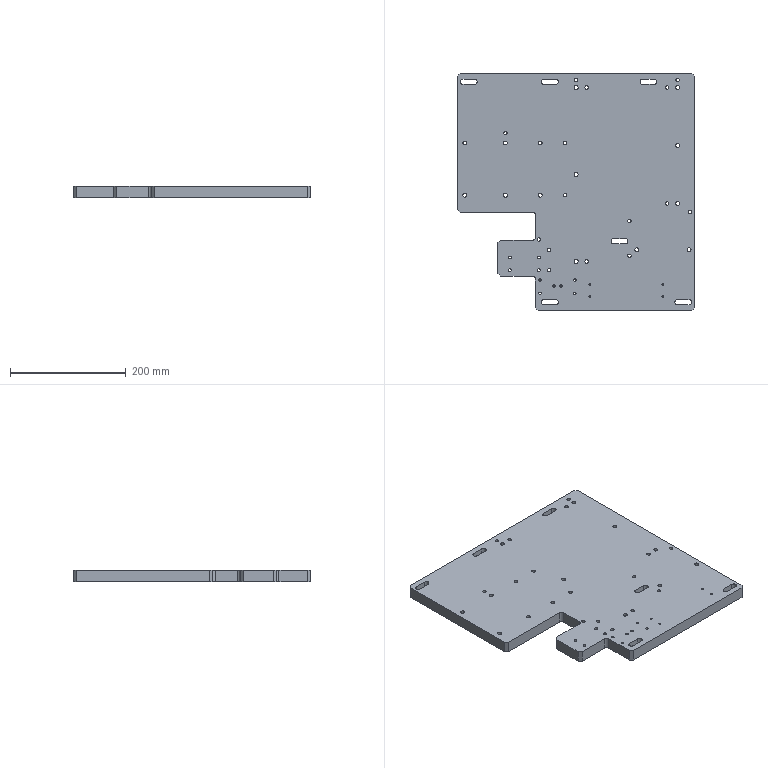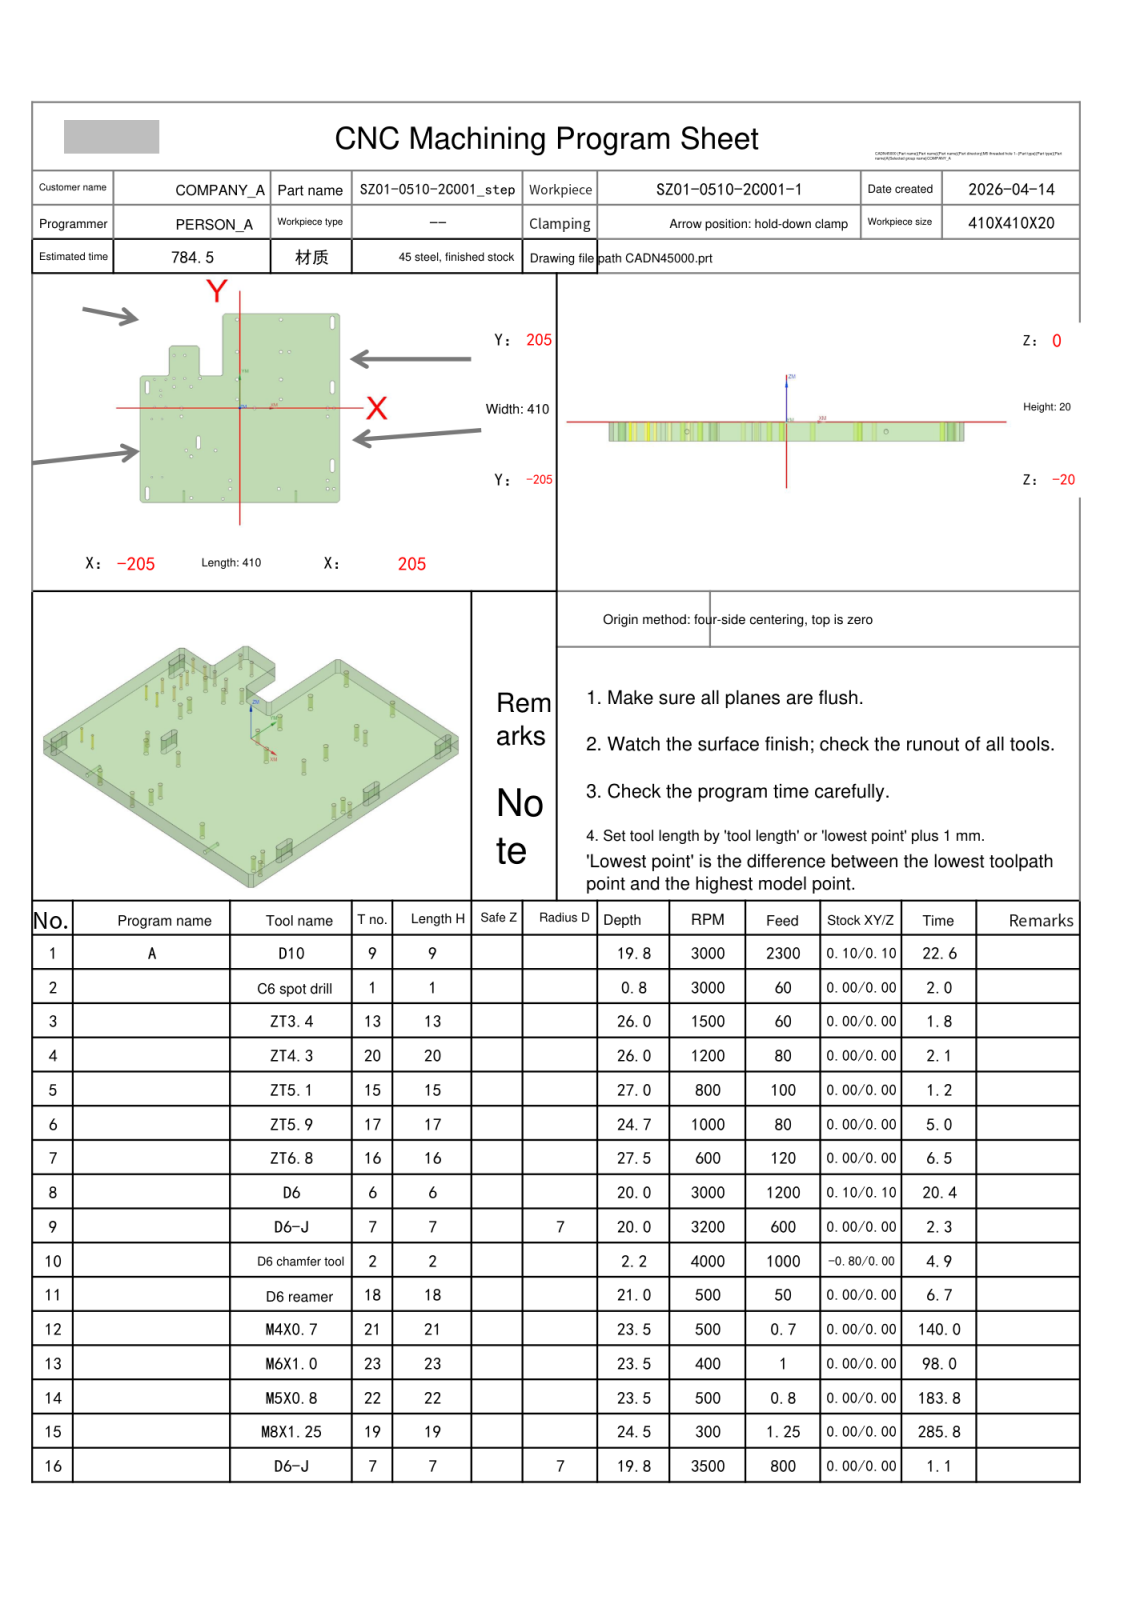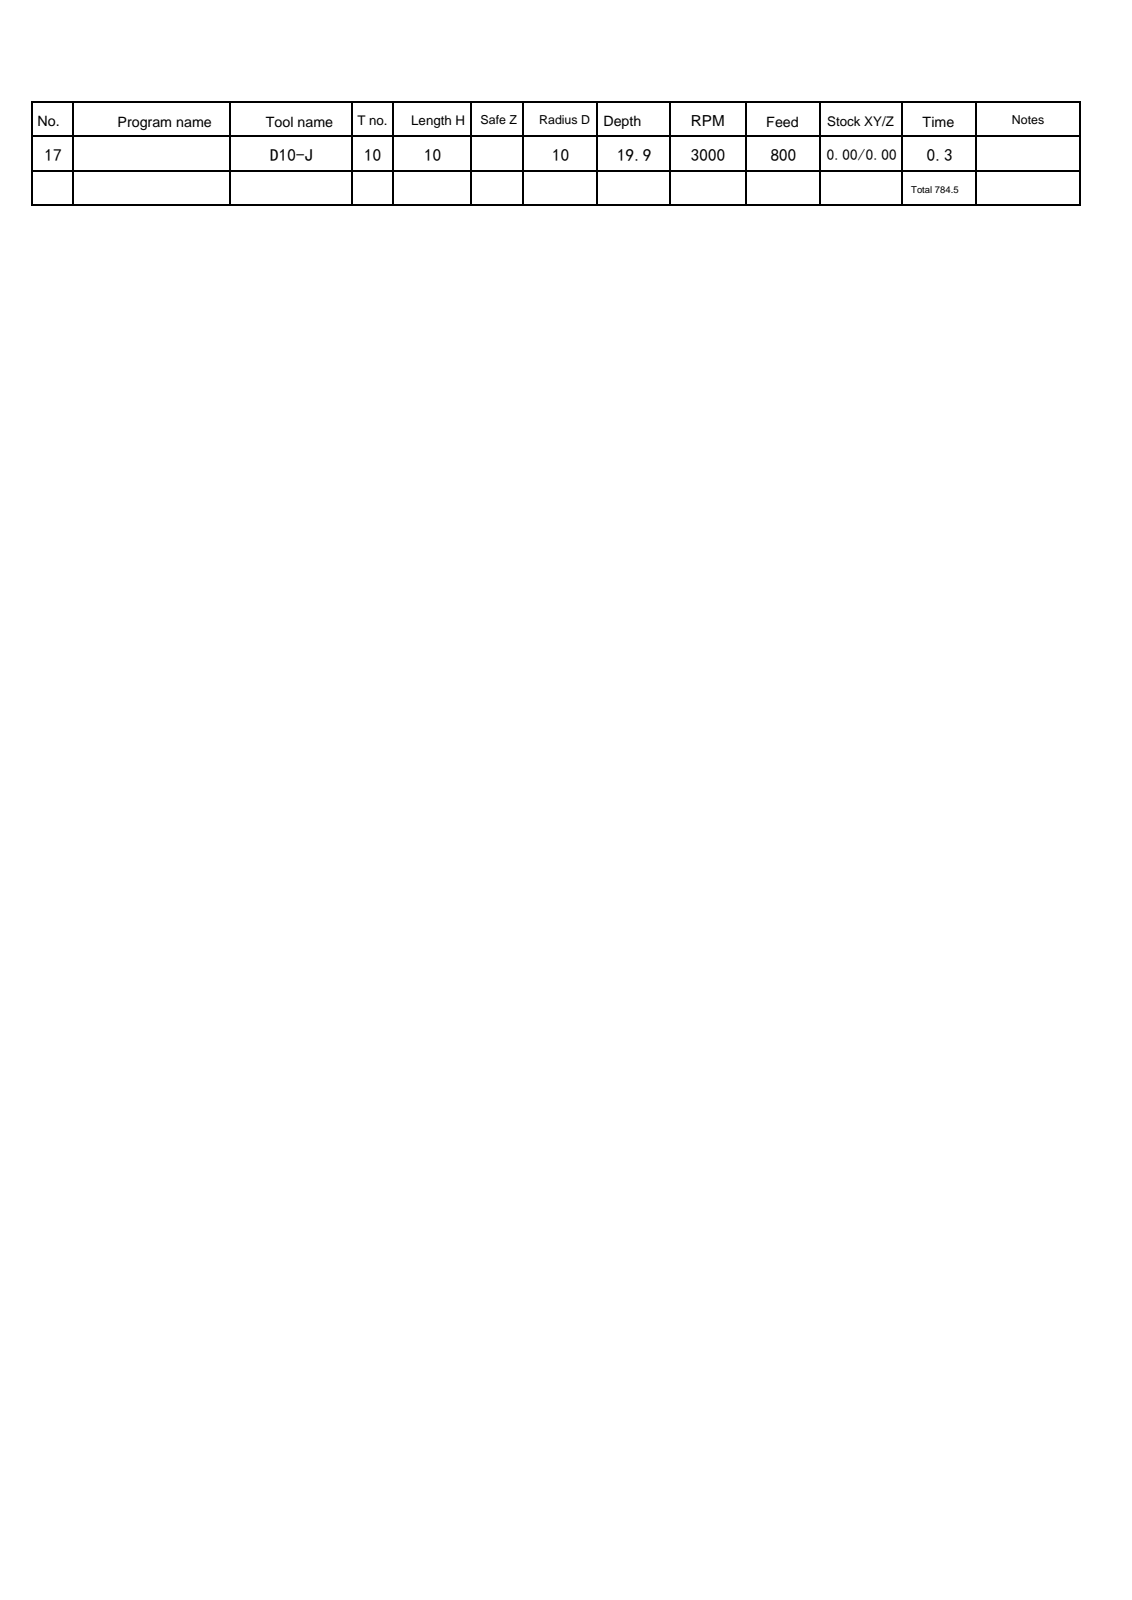NC program | NX | posted by the shop | part box 410 x 410 x 20 mm
Lines 26 to 1317 of 7905:
N1 T09 M06
(D10  D=10. R=0. H=09 ce=0.10 di=0.10)
G00 G90 G54 X215.1 Y-197.112 M03 S3000
G43 H09 Z50.
M08
Z-.2
G01 X208.606 Y-203.606 F2300.
X203.606 Y-208.606
X197.112 Y-215.1
G00 Z-.4
G01 X203.606 Y-208.606
X208.606 Y-203.606
X215.1 Y-197.112
G00 Z-.6
G01 X208.606 Y-203.606
X203.606 Y-208.606
X197.112 Y-215.1
G00 Z-.8
G01 X203.606 Y-208.606
X208.606 Y-203.606
X215.1 Y-197.112
G00 Z-1.
G01 X208.606 Y-203.606
X203.606 Y-208.606
X197.112 Y-215.1
G00 Z-1.2
G01 X203.606 Y-208.606
X208.606 Y-203.606
X215.1 Y-197.112
G00 Z-1.4
G01 X208.606 Y-203.606
X203.606 Y-208.606
X197.112 Y-215.1
G00 Z-1.6
G01 X203.606 Y-208.606
X208.606 Y-203.606
X215.1 Y-197.112
G00 Z-1.8
G01 X208.606 Y-203.606
X203.606 Y-208.606
X197.112 Y-215.1
G00 Z-2.
G01 X203.606 Y-208.606
X208.606 Y-203.606
X215.1 Y-197.112
G00 Z-2.2
G01 X208.606 Y-203.606
X203.606 Y-208.606
X197.112 Y-215.1
G00 Z-2.4
G01 X203.606 Y-208.606
X208.606 Y-203.606
X215.1 Y-197.112
G00 Z-2.6
G01 X208.606 Y-203.606
X203.606 Y-208.606
X197.112 Y-215.1
G00 Z-2.8
G01 X203.606 Y-208.606
X208.606 Y-203.606
X215.1 Y-197.112
G00 Z-3.
G01 X208.606 Y-203.606
X203.606 Y-208.606
X197.112 Y-215.1
G00 Z-3.2
G01 X203.606 Y-208.606
X208.606 Y-203.606
X215.1 Y-197.112
G00 Z-3.4
G01 X208.606 Y-203.606
X203.606 Y-208.606
X197.112 Y-215.1
G00 Z-3.6
G01 X203.606 Y-208.606
X208.606 Y-203.606
X215.1 Y-197.112
G00 Z-3.8
G01 X208.606 Y-203.606
X203.606 Y-208.606
X197.112 Y-215.1
G00 Z-4.
G01 X203.606 Y-208.606
X208.606 Y-203.606
X215.1 Y-197.112
G00 Z-4.2
G01 X208.606 Y-203.606
X203.606 Y-208.606
X197.112 Y-215.1
G00 Z-4.4
G01 X203.606 Y-208.606
X208.606 Y-203.606
X215.1 Y-197.112
G00 Z-4.6
G01 X208.606 Y-203.606
X203.606 Y-208.606
X197.112 Y-215.1
G00 Z-4.8
G01 X203.606 Y-208.606
X208.606 Y-203.606
X215.1 Y-197.112
G00 Z-5.
G01 X208.606 Y-203.606
X203.606 Y-208.606
X197.112 Y-215.1
G00 Z-5.2
G01 X203.606 Y-208.606
X208.606 Y-203.606
X215.1 Y-197.112
G00 Z-5.4
G01 X208.606 Y-203.606
X203.606 Y-208.606
X197.112 Y-215.1
G00 Z-5.6
G01 X203.606 Y-208.606
X208.606 Y-203.606
X215.1 Y-197.112
G00 Z-5.8
G01 X208.606 Y-203.606
X203.606 Y-208.606
X197.112 Y-215.1
G00 Z-6.
G01 X203.606 Y-208.606
X208.606 Y-203.606
X215.1 Y-197.112
G00 Z-6.2
G01 X208.606 Y-203.606
X203.606 Y-208.606
X197.112 Y-215.1
G00 Z-6.4
G01 X203.606 Y-208.606
X208.606 Y-203.606
X215.1 Y-197.112
G00 Z-6.6
G01 X208.606 Y-203.606
X203.606 Y-208.606
X197.112 Y-215.1
G00 Z-6.8
G01 X203.606 Y-208.606
X208.606 Y-203.606
X215.1 Y-197.112
G00 Z-7.
G01 X208.606 Y-203.606
X203.606 Y-208.606
X197.112 Y-215.1
G00 Z-7.2
G01 X203.606 Y-208.606
X208.606 Y-203.606
X215.1 Y-197.112
G00 Z-7.4
G01 X208.606 Y-203.606
X203.606 Y-208.606
X197.112 Y-215.1
G00 Z-7.6
G01 X203.606 Y-208.606
X208.606 Y-203.606
X215.1 Y-197.112
G00 Z-7.8
G01 X208.606 Y-203.606
X203.606 Y-208.606
X197.112 Y-215.1
G00 Z-8.
G01 X203.606 Y-208.606
X208.606 Y-203.606
X215.1 Y-197.112
G00 Z-8.2
G01 X208.606 Y-203.606
X203.606 Y-208.606
X197.112 Y-215.1
G00 Z-8.4
G01 X203.606 Y-208.606
X208.606 Y-203.606
X215.1 Y-197.112
G00 Z-8.6
G01 X208.606 Y-203.606
X203.606 Y-208.606
X197.112 Y-215.1
G00 Z-8.8
G01 X203.606 Y-208.606
X208.606 Y-203.606
X215.1 Y-197.112
G00 Z-9.
G01 X208.606 Y-203.606
X203.606 Y-208.606
X197.112 Y-215.1
G00 Z-9.2
G01 X203.606 Y-208.606
X208.606 Y-203.606
X215.1 Y-197.112
G00 Z-9.4
G01 X208.606 Y-203.606
X203.606 Y-208.606
X197.112 Y-215.1
G00 Z-9.6
G01 X203.606 Y-208.606
X208.606 Y-203.606
X215.1 Y-197.112
G00 Z-9.8
G01 X208.606 Y-203.606
X203.606 Y-208.606
X197.112 Y-215.1
G00 Z-10.
G01 X203.606 Y-208.606
X208.606 Y-203.606
X215.1 Y-197.112
G00 Z-10.2
G01 X208.606 Y-203.606
X203.606 Y-208.606
X197.112 Y-215.1
G00 Z-10.4
G01 X203.606 Y-208.606
X208.606 Y-203.606
X215.1 Y-197.112
G00 Z-10.6
G01 X208.606 Y-203.606
X203.606 Y-208.606
X197.112 Y-215.1
G00 Z-10.8
G01 X203.606 Y-208.606
X208.606 Y-203.606
X215.1 Y-197.112
G00 Z-11.
G01 X208.606 Y-203.606
X203.606 Y-208.606
X197.112 Y-215.1
G00 Z-11.2
G01 X203.606 Y-208.606
X208.606 Y-203.606
X215.1 Y-197.112
G00 Z-11.4
G01 X208.606 Y-203.606
X203.606 Y-208.606
X197.112 Y-215.1
G00 Z-11.6
G01 X203.606 Y-208.606
X208.606 Y-203.606
X215.1 Y-197.112
G00 Z-11.8
G01 X208.606 Y-203.606
X203.606 Y-208.606
X197.112 Y-215.1
G00 Z-12.
G01 X203.606 Y-208.606
X208.606 Y-203.606
X215.1 Y-197.112
G00 Z-12.2
G01 X208.606 Y-203.606
X203.606 Y-208.606
X197.112 Y-215.1
G00 Z-12.4
G01 X203.606 Y-208.606
X208.606 Y-203.606
X215.1 Y-197.112
G00 Z-12.6
G01 X208.606 Y-203.606
X203.606 Y-208.606
X197.112 Y-215.1
G00 Z-12.8
G01 X203.606 Y-208.606
X208.606 Y-203.606
X215.1 Y-197.112
G00 Z-13.
G01 X208.606 Y-203.606
X203.606 Y-208.606
X197.112 Y-215.1
G00 Z-13.2
G01 X203.606 Y-208.606
X208.606 Y-203.606
X215.1 Y-197.112
G00 Z-13.4
G01 X208.606 Y-203.606
X203.606 Y-208.606
X197.112 Y-215.1
G00 Z-13.6
G01 X203.606 Y-208.606
X208.606 Y-203.606
X215.1 Y-197.112
G00 Z-13.8
G01 X208.606 Y-203.606
X203.606 Y-208.606
X197.112 Y-215.1
G00 Z-14.
G01 X203.606 Y-208.606
X208.606 Y-203.606
X215.1 Y-197.112
G00 Z-14.2
G01 X208.606 Y-203.606
X203.606 Y-208.606
X197.112 Y-215.1
G00 Z-14.4
G01 X203.606 Y-208.606
X208.606 Y-203.606
X215.1 Y-197.112
G00 Z-14.6
G01 X208.606 Y-203.606
X203.606 Y-208.606
X197.112 Y-215.1
G00 Z-14.8
G01 X203.606 Y-208.606
X208.606 Y-203.606
X215.1 Y-197.112
G00 Z-15.
G01 X208.606 Y-203.606
X203.606 Y-208.606
X197.112 Y-215.1
G00 Z-15.2
G01 X203.606 Y-208.606
X208.606 Y-203.606
X215.1 Y-197.112
G00 Z-15.4
G01 X208.606 Y-203.606
X203.606 Y-208.606
X197.112 Y-215.1
G00 Z-15.6
G01 X203.606 Y-208.606
X208.606 Y-203.606
X215.1 Y-197.112
G00 Z-15.8
G01 X208.606 Y-203.606
X203.606 Y-208.606
X197.112 Y-215.1
G00 Z-16.
G01 X203.606 Y-208.606
X208.606 Y-203.606
X215.1 Y-197.112
G00 Z-16.2
G01 X208.606 Y-203.606
X203.606 Y-208.606
X197.112 Y-215.1
G00 Z-16.4
G01 X203.606 Y-208.606
X208.606 Y-203.606
X215.1 Y-197.112
G00 Z-16.6
G01 X208.606 Y-203.606
X203.606 Y-208.606
X197.112 Y-215.1
G00 Z-16.8
G01 X203.606 Y-208.606
X208.606 Y-203.606
X215.1 Y-197.112
G00 Z-17.
G01 X208.606 Y-203.606
X203.606 Y-208.606
X197.112 Y-215.1
G00 Z-17.2
G01 X203.606 Y-208.606
X208.606 Y-203.606
X215.1 Y-197.112
G00 Z-17.4
G01 X208.606 Y-203.606
X203.606 Y-208.606
X197.112 Y-215.1
G00 Z-17.6
G01 X203.606 Y-208.606
X208.606 Y-203.606
X215.1 Y-197.112
G00 Z-17.8
G01 X208.606 Y-203.606
X203.606 Y-208.606
X197.112 Y-215.1
G00 Z-18.
G01 X203.606 Y-208.606
X208.606 Y-203.606
X215.1 Y-197.112
G00 Z-18.2
G01 X208.606 Y-203.606
X203.606 Y-208.606
X197.112 Y-215.1
G00 Z-18.4
G01 X203.606 Y-208.606
X208.606 Y-203.606
X215.1 Y-197.112
G00 Z-18.6
G01 X208.606 Y-203.606
X203.606 Y-208.606
X197.112 Y-215.1
G00 Z-18.8
G01 X203.606 Y-208.606
X208.606 Y-203.606
X215.1 Y-197.112
G00 Z-19.
G01 X208.606 Y-203.606
X203.606 Y-208.606
X197.112 Y-215.1
G00 Z-19.2
G01 X203.606 Y-208.606
X208.606 Y-203.606
X215.1 Y-197.112
G00 Z-19.4
G01 X208.606 Y-203.606
X203.606 Y-208.606
X197.112 Y-215.1
G00 Z-19.6
G01 X203.606 Y-208.606
X208.606 Y-203.606
X215.1 Y-197.112
G00 Z-19.8
G01 X208.606 Y-203.606
X203.606 Y-208.606
X197.112 Y-215.1
G00 Z50.
X-197.112
Z-.2
G01 X-203.606 Y-208.606
X-208.606 Y-203.606
X-215.1 Y-197.112
G00 Z-.4
G01 X-208.606 Y-203.606
X-203.606 Y-208.606
X-197.112 Y-215.1
G00 Z-.6
G01 X-203.606 Y-208.606
X-208.606 Y-203.606
X-215.1 Y-197.112
G00 Z-.8
G01 X-208.606 Y-203.606
X-203.606 Y-208.606
X-197.112 Y-215.1
G00 Z-1.
G01 X-203.606 Y-208.606
X-208.606 Y-203.606
X-215.1 Y-197.112
G00 Z-1.2
G01 X-208.606 Y-203.606
X-203.606 Y-208.606
X-197.112 Y-215.1
G00 Z-1.4
G01 X-203.606 Y-208.606
X-208.606 Y-203.606
X-215.1 Y-197.112
G00 Z-1.6
G01 X-208.606 Y-203.606
X-203.606 Y-208.606
X-197.112 Y-215.1
G00 Z-1.8
G01 X-203.606 Y-208.606
X-208.606 Y-203.606
X-215.1 Y-197.112
G00 Z-2.
G01 X-208.606 Y-203.606
X-203.606 Y-208.606
X-197.112 Y-215.1
G00 Z-2.2
G01 X-203.606 Y-208.606
X-208.606 Y-203.606
X-215.1 Y-197.112
G00 Z-2.4
G01 X-208.606 Y-203.606
X-203.606 Y-208.606
X-197.112 Y-215.1
G00 Z-2.6
G01 X-203.606 Y-208.606
X-208.606 Y-203.606
X-215.1 Y-197.112
G00 Z-2.8
G01 X-208.606 Y-203.606
X-203.606 Y-208.606
X-197.112 Y-215.1
G00 Z-3.
G01 X-203.606 Y-208.606
X-208.606 Y-203.606
X-215.1 Y-197.112
G00 Z-3.2
G01 X-208.606 Y-203.606
X-203.606 Y-208.606
X-197.112 Y-215.1
G00 Z-3.4
G01 X-203.606 Y-208.606
X-208.606 Y-203.606
X-215.1 Y-197.112
G00 Z-3.6
G01 X-208.606 Y-203.606
X-203.606 Y-208.606
X-197.112 Y-215.1
G00 Z-3.8
G01 X-203.606 Y-208.606
X-208.606 Y-203.606
X-215.1 Y-197.112
G00 Z-4.
G01 X-208.606 Y-203.606
X-203.606 Y-208.606
X-197.112 Y-215.1
G00 Z-4.2
G01 X-203.606 Y-208.606
X-208.606 Y-203.606
X-215.1 Y-197.112
G00 Z-4.4
G01 X-208.606 Y-203.606
X-203.606 Y-208.606
X-197.112 Y-215.1
G00 Z-4.6
G01 X-203.606 Y-208.606
X-208.606 Y-203.606
X-215.1 Y-197.112
G00 Z-4.8
G01 X-208.606 Y-203.606
X-203.606 Y-208.606
X-197.112 Y-215.1
G00 Z-5.
G01 X-203.606 Y-208.606
X-208.606 Y-203.606
X-215.1 Y-197.112
G00 Z-5.2
G01 X-208.606 Y-203.606
X-203.606 Y-208.606
X-197.112 Y-215.1
G00 Z-5.4
G01 X-203.606 Y-208.606
X-208.606 Y-203.606
X-215.1 Y-197.112
G00 Z-5.6
G01 X-208.606 Y-203.606
X-203.606 Y-208.606
X-197.112 Y-215.1
G00 Z-5.8
G01 X-203.606 Y-208.606
X-208.606 Y-203.606
X-215.1 Y-197.112
G00 Z-6.
G01 X-208.606 Y-203.606
X-203.606 Y-208.606
X-197.112 Y-215.1
G00 Z-6.2
G01 X-203.606 Y-208.606
X-208.606 Y-203.606
X-215.1 Y-197.112
G00 Z-6.4
G01 X-208.606 Y-203.606
X-203.606 Y-208.606
X-197.112 Y-215.1
G00 Z-6.6
G01 X-203.606 Y-208.606
X-208.606 Y-203.606
X-215.1 Y-197.112
G00 Z-6.8
G01 X-208.606 Y-203.606
X-203.606 Y-208.606
X-197.112 Y-215.1
G00 Z-7.
G01 X-203.606 Y-208.606
X-208.606 Y-203.606
X-215.1 Y-197.112
G00 Z-7.2
G01 X-208.606 Y-203.606
X-203.606 Y-208.606
X-197.112 Y-215.1
G00 Z-7.4
G01 X-203.606 Y-208.606
X-208.606 Y-203.606
X-215.1 Y-197.112
G00 Z-7.6
G01 X-208.606 Y-203.606
X-203.606 Y-208.606
X-197.112 Y-215.1
G00 Z-7.8
G01 X-203.606 Y-208.606
X-208.606 Y-203.606
X-215.1 Y-197.112
G00 Z-8.
G01 X-208.606 Y-203.606
X-203.606 Y-208.606
X-197.112 Y-215.1
G00 Z-8.2
G01 X-203.606 Y-208.606
X-208.606 Y-203.606
X-215.1 Y-197.112
G00 Z-8.4
G01 X-208.606 Y-203.606
X-203.606 Y-208.606
X-197.112 Y-215.1
G00 Z-8.6
G01 X-203.606 Y-208.606
X-208.606 Y-203.606
X-215.1 Y-197.112
G00 Z-8.8
G01 X-208.606 Y-203.606
X-203.606 Y-208.606
X-197.112 Y-215.1
G00 Z-9.
G01 X-203.606 Y-208.606
X-208.606 Y-203.606
X-215.1 Y-197.112
G00 Z-9.2
G01 X-208.606 Y-203.606
X-203.606 Y-208.606
X-197.112 Y-215.1
G00 Z-9.4
G01 X-203.606 Y-208.606
X-208.606 Y-203.606
X-215.1 Y-197.112
G00 Z-9.6
G01 X-208.606 Y-203.606
X-203.606 Y-208.606
X-197.112 Y-215.1
G00 Z-9.8
G01 X-203.606 Y-208.606
X-208.606 Y-203.606
X-215.1 Y-197.112
G00 Z-10.
G01 X-208.606 Y-203.606
X-203.606 Y-208.606
X-197.112 Y-215.1
G00 Z-10.2
G01 X-203.606 Y-208.606
X-208.606 Y-203.606
X-215.1 Y-197.112
G00 Z-10.4
G01 X-208.606 Y-203.606
X-203.606 Y-208.606
X-197.112 Y-215.1
G00 Z-10.6
G01 X-203.606 Y-208.606
X-208.606 Y-203.606
X-215.1 Y-197.112
G00 Z-10.8
G01 X-208.606 Y-203.606
X-203.606 Y-208.606
X-197.112 Y-215.1
G00 Z-11.
G01 X-203.606 Y-208.606
X-208.606 Y-203.606
X-215.1 Y-197.112
G00 Z-11.2
G01 X-208.606 Y-203.606
X-203.606 Y-208.606
X-197.112 Y-215.1
G00 Z-11.4
G01 X-203.606 Y-208.606
X-208.606 Y-203.606
X-215.1 Y-197.112
G00 Z-11.6
G01 X-208.606 Y-203.606
X-203.606 Y-208.606
X-197.112 Y-215.1
G00 Z-11.8
G01 X-203.606 Y-208.606
X-208.606 Y-203.606
X-215.1 Y-197.112
G00 Z-12.
G01 X-208.606 Y-203.606
X-203.606 Y-208.606
X-197.112 Y-215.1
G00 Z-12.2
G01 X-203.606 Y-208.606
X-208.606 Y-203.606
X-215.1 Y-197.112
G00 Z-12.4
G01 X-208.606 Y-203.606
X-203.606 Y-208.606
X-197.112 Y-215.1
G00 Z-12.6
G01 X-203.606 Y-208.606
X-208.606 Y-203.606
X-215.1 Y-197.112
G00 Z-12.8
G01 X-208.606 Y-203.606
X-203.606 Y-208.606
X-197.112 Y-215.1
G00 Z-13.
G01 X-203.606 Y-208.606
X-208.606 Y-203.606
X-215.1 Y-197.112
G00 Z-13.2
G01 X-208.606 Y-203.606
X-203.606 Y-208.606
X-197.112 Y-215.1
G00 Z-13.4
G01 X-203.606 Y-208.606
X-208.606 Y-203.606
X-215.1 Y-197.112
G00 Z-13.6
G01 X-208.606 Y-203.606
X-203.606 Y-208.606
X-197.112 Y-215.1
G00 Z-13.8
G01 X-203.606 Y-208.606
X-208.606 Y-203.606
X-215.1 Y-197.112
G00 Z-14.
G01 X-208.606 Y-203.606
X-203.606 Y-208.606
X-197.112 Y-215.1
G00 Z-14.2
G01 X-203.606 Y-208.606
X-208.606 Y-203.606
X-215.1 Y-197.112
G00 Z-14.4
G01 X-208.606 Y-203.606
X-203.606 Y-208.606
X-197.112 Y-215.1
G00 Z-14.6
G01 X-203.606 Y-208.606
X-208.606 Y-203.606
X-215.1 Y-197.112
G00 Z-14.8
G01 X-208.606 Y-203.606
X-203.606 Y-208.606
X-197.112 Y-215.1
G00 Z-15.
G01 X-203.606 Y-208.606
X-208.606 Y-203.606
X-215.1 Y-197.112
G00 Z-15.2
G01 X-208.606 Y-203.606
X-203.606 Y-208.606
X-197.112 Y-215.1
G00 Z-15.4
G01 X-203.606 Y-208.606
X-208.606 Y-203.606
X-215.1 Y-197.112
G00 Z-15.6
G01 X-208.606 Y-203.606
X-203.606 Y-208.606
X-197.112 Y-215.1
G00 Z-15.8
G01 X-203.606 Y-208.606
X-208.606 Y-203.606
X-215.1 Y-197.112
G00 Z-16.
G01 X-208.606 Y-203.606
X-203.606 Y-208.606
X-197.112 Y-215.1
G00 Z-16.2
G01 X-203.606 Y-208.606
X-208.606 Y-203.606
X-215.1 Y-197.112
G00 Z-16.4
G01 X-208.606 Y-203.606
X-203.606 Y-208.606
X-197.112 Y-215.1
G00 Z-16.6
G01 X-203.606 Y-208.606
X-208.606 Y-203.606
X-215.1 Y-197.112
G00 Z-16.8
G01 X-208.606 Y-203.606
X-203.606 Y-208.606
X-197.112 Y-215.1
G00 Z-17.
G01 X-203.606 Y-208.606
X-208.606 Y-203.606
X-215.1 Y-197.112
G00 Z-17.2
G01 X-208.606 Y-203.606
X-203.606 Y-208.606
X-197.112 Y-215.1
G00 Z-17.4
G01 X-203.606 Y-208.606
X-208.606 Y-203.606
X-215.1 Y-197.112
G00 Z-17.6
G01 X-208.606 Y-203.606
X-203.606 Y-208.606
X-197.112 Y-215.1
G00 Z-17.8
G01 X-203.606 Y-208.606
X-208.606 Y-203.606
X-215.1 Y-197.112
G00 Z-18.
G01 X-208.606 Y-203.606
X-203.606 Y-208.606
X-197.112 Y-215.1
G00 Z-18.2
G01 X-203.606 Y-208.606
X-208.606 Y-203.606
X-215.1 Y-197.112
G00 Z-18.4
G01 X-208.606 Y-203.606
X-203.606 Y-208.606
X-197.112 Y-215.1
G00 Z-18.6
G01 X-203.606 Y-208.606
X-208.606 Y-203.606
X-215.1 Y-197.112
G00 Z-18.8
G01 X-208.606 Y-203.606
X-203.606 Y-208.606
X-197.112 Y-215.1
G00 Z-19.
G01 X-203.606 Y-208.606
X-208.606 Y-203.606
X-215.1 Y-197.112
G00 Z-19.2
G01 X-208.606 Y-203.606
X-203.606 Y-208.606
X-197.112 Y-215.1
G00 Z-19.4
G01 X-203.606 Y-208.606
X-208.606 Y-203.606
X-215.1 Y-197.112
G00 Z-19.6
G01 X-208.606 Y-203.606
X-203.606 Y-208.606
X-197.112 Y-215.1
G00 Z-19.8
G01 X-203.606 Y-208.606
X-208.606 Y-203.606
X-215.1 Y-197.112
G00 Z50.
Y62.112
Z-.2
G01 X-208.606 Y68.606
X-203.606 Y73.606
G02 X-200. Y75.1 I3.606 J-3.606
G01 X-150.1
Y130.
G02 X-148.606 Y133.606 I5.1 J0.0
G01 X-143.606 Y138.606
G02 X-140. Y140.1 I3.606 J-3.606
G01 X-88.
G02 X-84.394 Y138.606 I0.0 J-5.1
G01 X-79.394 Y133.606
G02 X-77.9 Y130. I-3.606 J-3.606
G01 Y75.1
X-40.1
Y200.
G02 X-38.606 Y203.606 I5.1 J0.0
G01 X-33.606 Y208.606
X-27.112 Y215.1
G00 Z-.4
G01 X-33.606 Y208.606
X-38.606 Y203.606
G03 X-40.1 Y200. I3.606 J-3.606
G01 Y75.1
X-77.9
Y130.
G03 X-79.394 Y133.606 I-5.1 J0.0
G01 X-84.394 Y138.606
G03 X-88. Y140.1 I-3.606 J-3.606
G01 X-140.
G03 X-143.606 Y138.606 I0.0 J-5.1
G01 X-148.606 Y133.606
G03 X-150.1 Y130. I3.606 J-3.606
G01 Y75.1
X-200.
G03 X-203.606 Y73.606 I0.0 J-5.1
G01 X-208.606 Y68.606
X-215.1 Y62.112
G00 Z-.6
G01 X-208.606 Y68.606
X-203.606 Y73.606
G02 X-200. Y75.1 I3.606 J-3.606
G01 X-150.1
Y130.
G02 X-148.606 Y133.606 I5.1 J0.0
G01 X-143.606 Y138.606
G02 X-140. Y140.1 I3.606 J-3.606
G01 X-88.
G02 X-84.394 Y138.606 I0.0 J-5.1
G01 X-79.394 Y133.606
G02 X-77.9 Y130. I-3.606 J-3.606
G01 Y75.1
X-40.1
Y200.
G02 X-38.606 Y203.606 I5.1 J0.0
G01 X-33.606 Y208.606
X-27.112 Y215.1
G00 Z-.8
G01 X-33.606 Y208.606
X-38.606 Y203.606
G03 X-40.1 Y200. I3.606 J-3.606
G01 Y75.1
X-77.9
Y130.
G03 X-79.394 Y133.606 I-5.1 J0.0
G01 X-84.394 Y138.606
G03 X-88. Y140.1 I-3.606 J-3.606
G01 X-140.
G03 X-143.606 Y138.606 I0.0 J-5.1
G01 X-148.606 Y133.606
G03 X-150.1 Y130. I3.606 J-3.606
G01 Y75.1
X-200.
G03 X-203.606 Y73.606 I0.0 J-5.1
G01 X-208.606 Y68.606
X-215.1 Y62.112
G00 Z-1.
G01 X-208.606 Y68.606
X-203.606 Y73.606
G02 X-200. Y75.1 I3.606 J-3.606
G01 X-150.1
Y130.
G02 X-148.606 Y133.606 I5.1 J0.0
G01 X-143.606 Y138.606
G02 X-140. Y140.1 I3.606 J-3.606
G01 X-88.
G02 X-84.394 Y138.606 I0.0 J-5.1
G01 X-79.394 Y133.606
G02 X-77.9 Y130. I-3.606 J-3.606
G01 Y75.1
X-40.1
Y200.
G02 X-38.606 Y203.606 I5.1 J0.0
G01 X-33.606 Y208.606
X-27.112 Y215.1
G00 Z-1.2
G01 X-33.606 Y208.606
X-38.606 Y203.606
G03 X-40.1 Y200. I3.606 J-3.606
G01 Y75.1
X-77.9
Y130.
G03 X-79.394 Y133.606 I-5.1 J0.0
G01 X-84.394 Y138.606
G03 X-88. Y140.1 I-3.606 J-3.606
G01 X-140.
G03 X-143.606 Y138.606 I0.0 J-5.1
G01 X-148.606 Y133.606
G03 X-150.1 Y130. I3.606 J-3.606
G01 Y75.1
X-200.
G03 X-203.606 Y73.606 I0.0 J-5.1
G01 X-208.606 Y68.606
X-215.1 Y62.112
G00 Z-1.4
G01 X-208.606 Y68.606
X-203.606 Y73.606
G02 X-200. Y75.1 I3.606 J-3.606
G01 X-150.1
Y130.
G02 X-148.606 Y133.606 I5.1 J0.0
G01 X-143.606 Y138.606
G02 X-140. Y140.1 I3.606 J-3.606
G01 X-88.
G02 X-84.394 Y138.606 I0.0 J-5.1
G01 X-79.394 Y133.606
G02 X-77.9 Y130. I-3.606 J-3.606
G01 Y75.1
X-40.1
Y200.
G02 X-38.606 Y203.606 I5.1 J0.0
G01 X-33.606 Y208.606
X-27.112 Y215.1
G00 Z-1.6
G01 X-33.606 Y208.606
X-38.606 Y203.606
G03 X-40.1 Y200. I3.606 J-3.606
G01 Y75.1
X-77.9
Y130.
G03 X-79.394 Y133.606 I-5.1 J0.0
G01 X-84.394 Y138.606
G03 X-88. Y140.1 I-3.606 J-3.606
G01 X-140.
G03 X-143.606 Y138.606 I0.0 J-5.1
G01 X-148.606 Y133.606
G03 X-150.1 Y130. I3.606 J-3.606
G01 Y75.1
X-200.
G03 X-203.606 Y73.606 I0.0 J-5.1
G01 X-208.606 Y68.606
X-215.1 Y62.112
G00 Z-1.8
G01 X-208.606 Y68.606
X-203.606 Y73.606
G02 X-200. Y75.1 I3.606 J-3.606
G01 X-150.1
Y130.
G02 X-148.606 Y133.606 I5.1 J0.0
G01 X-143.606 Y138.606
G02 X-140. Y140.1 I3.606 J-3.606
G01 X-88.
G02 X-84.394 Y138.606 I0.0 J-5.1
G01 X-79.394 Y133.606
G02 X-77.9 Y130. I-3.606 J-3.606
G01 Y75.1
X-40.1
Y200.
G02 X-38.606 Y203.606 I5.1 J0.0
G01 X-33.606 Y208.606
X-27.112 Y215.1
G00 Z-2.
G01 X-33.606 Y208.606
X-38.606 Y203.606
G03 X-40.1 Y200. I3.606 J-3.606
G01 Y75.1
X-77.9
Y130.
G03 X-79.394 Y133.606 I-5.1 J0.0
G01 X-84.394 Y138.606
G03 X-88. Y140.1 I-3.606 J-3.606
G01 X-140.
G03 X-143.606 Y138.606 I0.0 J-5.1
G01 X-148.606 Y133.606
G03 X-150.1 Y130. I3.606 J-3.606
G01 Y75.1
X-200.
G03 X-203.606 Y73.606 I0.0 J-5.1
G01 X-208.606 Y68.606
X-215.1 Y62.112
G00 Z-2.2
G01 X-208.606 Y68.606
X-203.606 Y73.606
G02 X-200. Y75.1 I3.606 J-3.606
G01 X-150.1
Y130.
G02 X-148.606 Y133.606 I5.1 J0.0
G01 X-143.606 Y138.606
G02 X-140. Y140.1 I3.606 J-3.606
G01 X-88.
G02 X-84.394 Y138.606 I0.0 J-5.1
G01 X-79.394 Y133.606
G02 X-77.9 Y130. I-3.606 J-3.606
G01 Y75.1
X-40.1
Y200.
G02 X-38.606 Y203.606 I5.1 J0.0
G01 X-33.606 Y208.606
X-27.112 Y215.1
G00 Z-2.4
G01 X-33.606 Y208.606
X-38.606 Y203.606
G03 X-40.1 Y200. I3.606 J-3.606
G01 Y75.1
X-77.9
Y130.
G03 X-79.394 Y133.606 I-5.1 J0.0
G01 X-84.394 Y138.606
G03 X-88. Y140.1 I-3.606 J-3.606
G01 X-140.
G03 X-143.606 Y138.606 I0.0 J-5.1
G01 X-148.606 Y133.606
G03 X-150.1 Y130. I3.606 J-3.606
G01 Y75.1
X-200.
G03 X-203.606 Y73.606 I0.0 J-5.1
G01 X-208.606 Y68.606
X-215.1 Y62.112
G00 Z-2.6
G01 X-208.606 Y68.606
X-203.606 Y73.606
G02 X-200. Y75.1 I3.606 J-3.606
G01 X-150.1
Y130.
G02 X-148.606 Y133.606 I5.1 J0.0
G01 X-143.606 Y138.606
G02 X-140. Y140.1 I3.606 J-3.606
G01 X-88.
G02 X-84.394 Y138.606 I0.0 J-5.1
G01 X-79.394 Y133.606
G02 X-77.9 Y130. I-3.606 J-3.606
G01 Y75.1
X-40.1
Y200.
G02 X-38.606 Y203.606 I5.1 J0.0
G01 X-33.606 Y208.606
X-27.112 Y215.1
G00 Z-2.8
G01 X-33.606 Y208.606
X-38.606 Y203.606
G03 X-40.1 Y200. I3.606 J-3.606
G01 Y75.1
X-77.9
Y130.
G03 X-79.394 Y133.606 I-5.1 J0.0
G01 X-84.394 Y138.606
G03 X-88. Y140.1 I-3.606 J-3.606
G01 X-140.
G03 X-143.606 Y138.606 I0.0 J-5.1
G01 X-148.606 Y133.606
G03 X-150.1 Y130. I3.606 J-3.606
G01 Y75.1
X-200.
G03 X-203.606 Y73.606 I0.0 J-5.1
G01 X-208.606 Y68.606
X-215.1 Y62.112
G00 Z-3.
G01 X-208.606 Y68.606
X-203.606 Y73.606
G02 X-200. Y75.1 I3.606 J-3.606
G01 X-150.1
Y130.
G02 X-148.606 Y133.606 I5.1 J0.0
G01 X-143.606 Y138.606
G02 X-140. Y140.1 I3.606 J-3.606
G01 X-88.
G02 X-84.394 Y138.606 I0.0 J-5.1
G01 X-79.394 Y133.606
G02 X-77.9 Y130. I-3.606 J-3.606
G01 Y75.1
X-40.1
Y200.
G02 X-38.606 Y203.606 I5.1 J0.0
G01 X-33.606 Y208.606
X-27.112 Y215.1
G00 Z-3.2
G01 X-33.606 Y208.606
X-38.606 Y203.606
G03 X-40.1 Y200. I3.606 J-3.606
G01 Y75.1
X-77.9
Y130.
G03 X-79.394 Y133.606 I-5.1 J0.0
G01 X-84.394 Y138.606
G03 X-88. Y140.1 I-3.606 J-3.606
G01 X-140.
G03 X-143.606 Y138.606 I0.0 J-5.1
G01 X-148.606 Y133.606
G03 X-150.1 Y130. I3.606 J-3.606
G01 Y75.1
X-200.
G03 X-203.606 Y73.606 I0.0 J-5.1
G01 X-208.606 Y68.606
X-215.1 Y62.112
G00 Z-3.4
G01 X-208.606 Y68.606
X-203.606 Y73.606
G02 X-200. Y75.1 I3.606 J-3.606
G01 X-150.1
Y130.
G02 X-148.606 Y133.606 I5.1 J0.0
G01 X-143.606 Y138.606
G02 X-140. Y140.1 I3.606 J-3.606
G01 X-88.
G02 X-84.394 Y138.606 I0.0 J-5.1
G01 X-79.394 Y133.606
G02 X-77.9 Y130. I-3.606 J-3.606
G01 Y75.1
X-40.1
Y200.
G02 X-38.606 Y203.606 I5.1 J0.0
G01 X-33.606 Y208.606
X-27.112 Y215.1
G00 Z-3.6
G01 X-33.606 Y208.606
X-38.606 Y203.606
G03 X-40.1 Y200. I3.606 J-3.606
G01 Y75.1
X-77.9
Y130.
G03 X-79.394 Y133.606 I-5.1 J0.0
G01 X-84.394 Y138.606
G03 X-88. Y140.1 I-3.606 J-3.606
G01 X-140.
G03 X-143.606 Y138.606 I0.0 J-5.1
G01 X-148.606 Y133.606
G03 X-150.1 Y130. I3.606 J-3.606
G01 Y75.1
X-200.
G03 X-203.606 Y73.606 I0.0 J-5.1
G01 X-208.606 Y68.606
X-215.1 Y62.112
G00 Z-3.8
G01 X-208.606 Y68.606
X-203.606 Y73.606
G02 X-200. Y75.1 I3.606 J-3.606
G01 X-150.1
Y130.
G02 X-148.606 Y133.606 I5.1 J0.0
G01 X-143.606 Y138.606
G02 X-140. Y140.1 I3.606 J-3.606
G01 X-88.
G02 X-84.394 Y138.606 I0.0 J-5.1
G01 X-79.394 Y133.606
G02 X-77.9 Y130. I-3.606 J-3.606
G01 Y75.1
X-40.1
Y200.
G02 X-38.606 Y203.606 I5.1 J0.0
G01 X-33.606 Y208.606
X-27.112 Y215.1
G00 Z-4.
G01 X-33.606 Y208.606
X-38.606 Y203.606
G03 X-40.1 Y200. I3.606 J-3.606
G01 Y75.1
X-77.9
Y130.
G03 X-79.394 Y133.606 I-5.1 J0.0
G01 X-84.394 Y138.606
G03 X-88. Y140.1 I-3.606 J-3.606
G01 X-140.
G03 X-143.606 Y138.606 I0.0 J-5.1
G01 X-148.606 Y133.606
G03 X-150.1 Y130. I3.606 J-3.606
G01 Y75.1
X-200.
G03 X-203.606 Y73.606 I0.0 J-5.1
G01 X-208.606 Y68.606
X-215.1 Y62.112
G00 Z-4.2
G01 X-208.606 Y68.606
X-203.606 Y73.606
G02 X-200. Y75.1 I3.606 J-3.606
G01 X-150.1
Y130.
G02 X-148.606 Y133.606 I5.1 J0.0
G01 X-143.606 Y138.606
G02 X-140. Y140.1 I3.606 J-3.606
G01 X-88.
G02 X-84.394 Y138.606 I0.0 J-5.1
G01 X-79.394 Y133.606
G02 X-77.9 Y130. I-3.606 J-3.606
G01 Y75.1
X-40.1
Y200.
G02 X-38.606 Y203.606 I5.1 J0.0
G01 X-33.606 Y208.606
X-27.112 Y215.1
G00 Z-4.4
G01 X-33.606 Y208.606
X-38.606 Y203.606
G03 X-40.1 Y200. I3.606 J-3.606
G01 Y75.1
X-77.9
Y130.
G03 X-79.394 Y133.606 I-5.1 J0.0
G01 X-84.394 Y138.606
G03 X-88. Y140.1 I-3.606 J-3.606
G01 X-140.
G03 X-143.606 Y138.606 I0.0 J-5.1
G01 X-148.606 Y133.606
G03 X-150.1 Y130. I3.606 J-3.606
G01 Y75.1
X-200.
G03 X-203.606 Y73.606 I0.0 J-5.1
G01 X-208.606 Y68.606
X-215.1 Y62.112
G00 Z-4.6
G01 X-208.606 Y68.606
X-203.606 Y73.606
G02 X-200. Y75.1 I3.606 J-3.606
G01 X-150.1
Y130.
G02 X-148.606 Y133.606 I5.1 J0.0
G01 X-143.606 Y138.606
G02 X-140. Y140.1 I3.606 J-3.606
G01 X-88.
G02 X-84.394 Y138.606 I0.0 J-5.1
G01 X-79.394 Y133.606
G02 X-77.9 Y130. I-3.606 J-3.606
G01 Y75.1
X-40.1
Y200.
G02 X-38.606 Y203.606 I5.1 J0.0
G01 X-33.606 Y208.606
X-27.112 Y215.1
G00 Z-4.8
G01 X-33.606 Y208.606
X-38.606 Y203.606
G03 X-40.1 Y200. I3.606 J-3.606
G01 Y75.1
X-77.9
Y130.
G03 X-79.394 Y133.606 I-5.1 J0.0
G01 X-84.394 Y138.606
G03 X-88. Y140.1 I-3.606 J-3.606
G01 X-140.
G03 X-143.606 Y138.606 I0.0 J-5.1
G01 X-148.606 Y133.606
G03 X-150.1 Y130. I3.606 J-3.606
G01 Y75.1
X-200.
G03 X-203.606 Y73.606 I0.0 J-5.1
G01 X-208.606 Y68.606
X-215.1 Y62.112
G00 Z-5.
G01 X-208.606 Y68.606
X-203.606 Y73.606
G02 X-200. Y75.1 I3.606 J-3.606
G01 X-150.1
Y130.
G02 X-148.606 Y133.606 I5.1 J0.0
G01 X-143.606 Y138.606
G02 X-140. Y140.1 I3.606 J-3.606
G01 X-88.
G02 X-84.394 Y138.606 I0.0 J-5.1
G01 X-79.394 Y133.606
G02 X-77.9 Y130. I-3.606 J-3.606
G01 Y75.1
X-40.1
Y200.
G02 X-38.606 Y203.606 I5.1 J0.0
G01 X-33.606 Y208.606
X-27.112 Y215.1
G00 Z-5.2
G01 X-33.606 Y208.606
X-38.606 Y203.606
G03 X-40.1 Y200. I3.606 J-3.606
G01 Y75.1
X-77.9
Y130.
G03 X-79.394 Y133.606 I-5.1 J0.0
G01 X-84.394 Y138.606
G03 X-88. Y140.1 I-3.606 J-3.606
G01 X-140.
G03 X-143.606 Y138.606 I0.0 J-5.1
G01 X-148.606 Y133.606
G03 X-150.1 Y130. I3.606 J-3.606
G01 Y75.1
X-200.